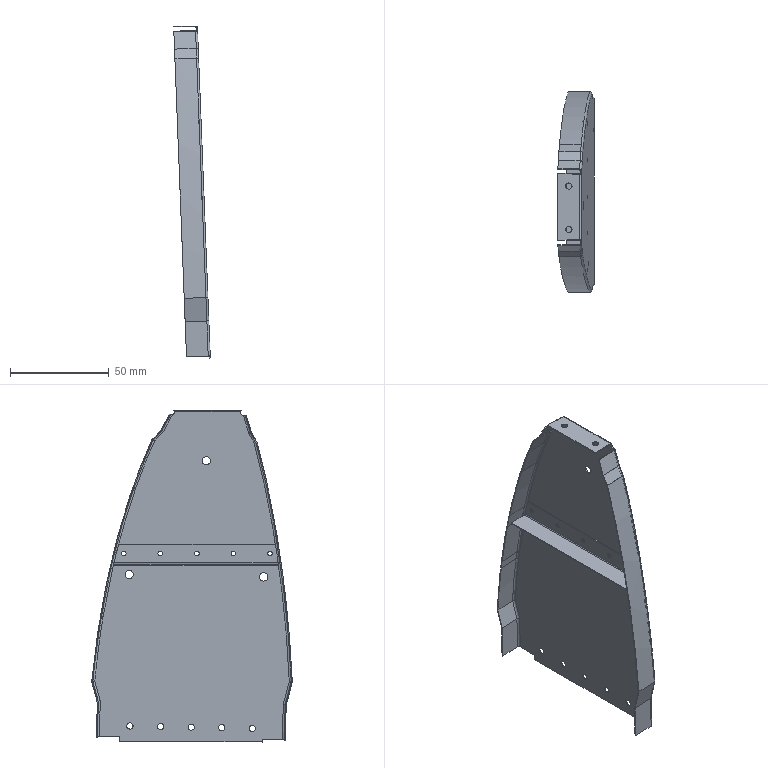Part | SolidWorks | features BaseBody 2 | 2 solids | 131 faces | box 18.494 x 101.443 x 167.963 mm | volume 9710 mm3 | cylinder 58 | plane 39 | spline 34 | commonest cylinder face diameters 2 x28 2.4 x20 1 x2 4.119 x2 4.151 x2 4.287 x2